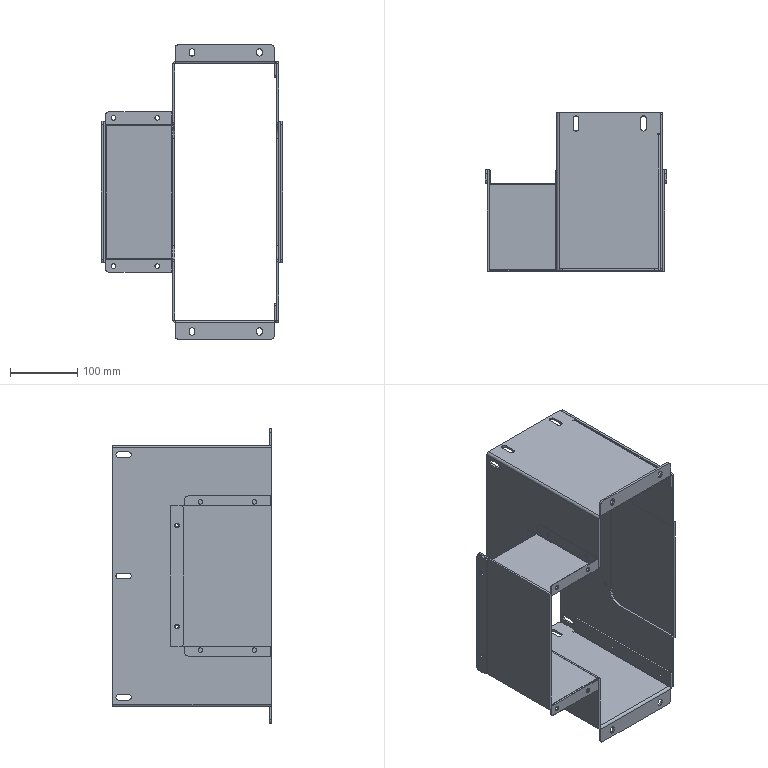Part | SolidWorks | features AEMSimFeature 1 | 7 solids | 346 faces | box 269 x 235 x 437 mm | volume 927122 mm3 | plane 180 | cylinder 162 | spline 4 | commonest cylinder face diameters 8 x40 7 x34 10 x20 5 x16 1 x14 6 x14